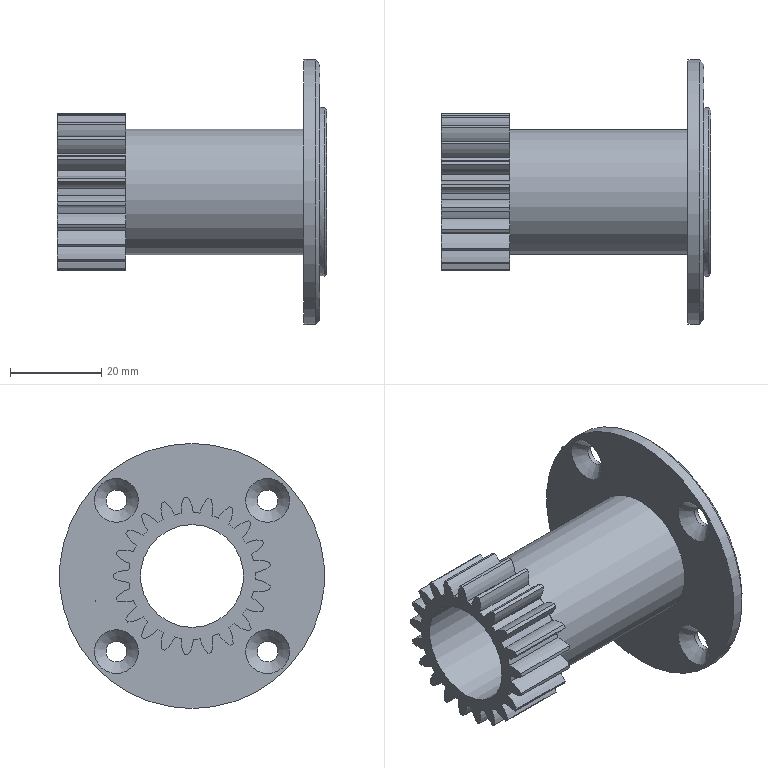Part | NX | features BREP 1 | 1 solid | 107 faces | box 59 x 58 x 58 mm | volume 20572 mm3 | cylinder 94 | cone 7 | plane 6 | commonest cylinder face diameters 12.6 x42 27.748 x21 34.55 x21 4.5 x4 0.1 x1 22.5 x1